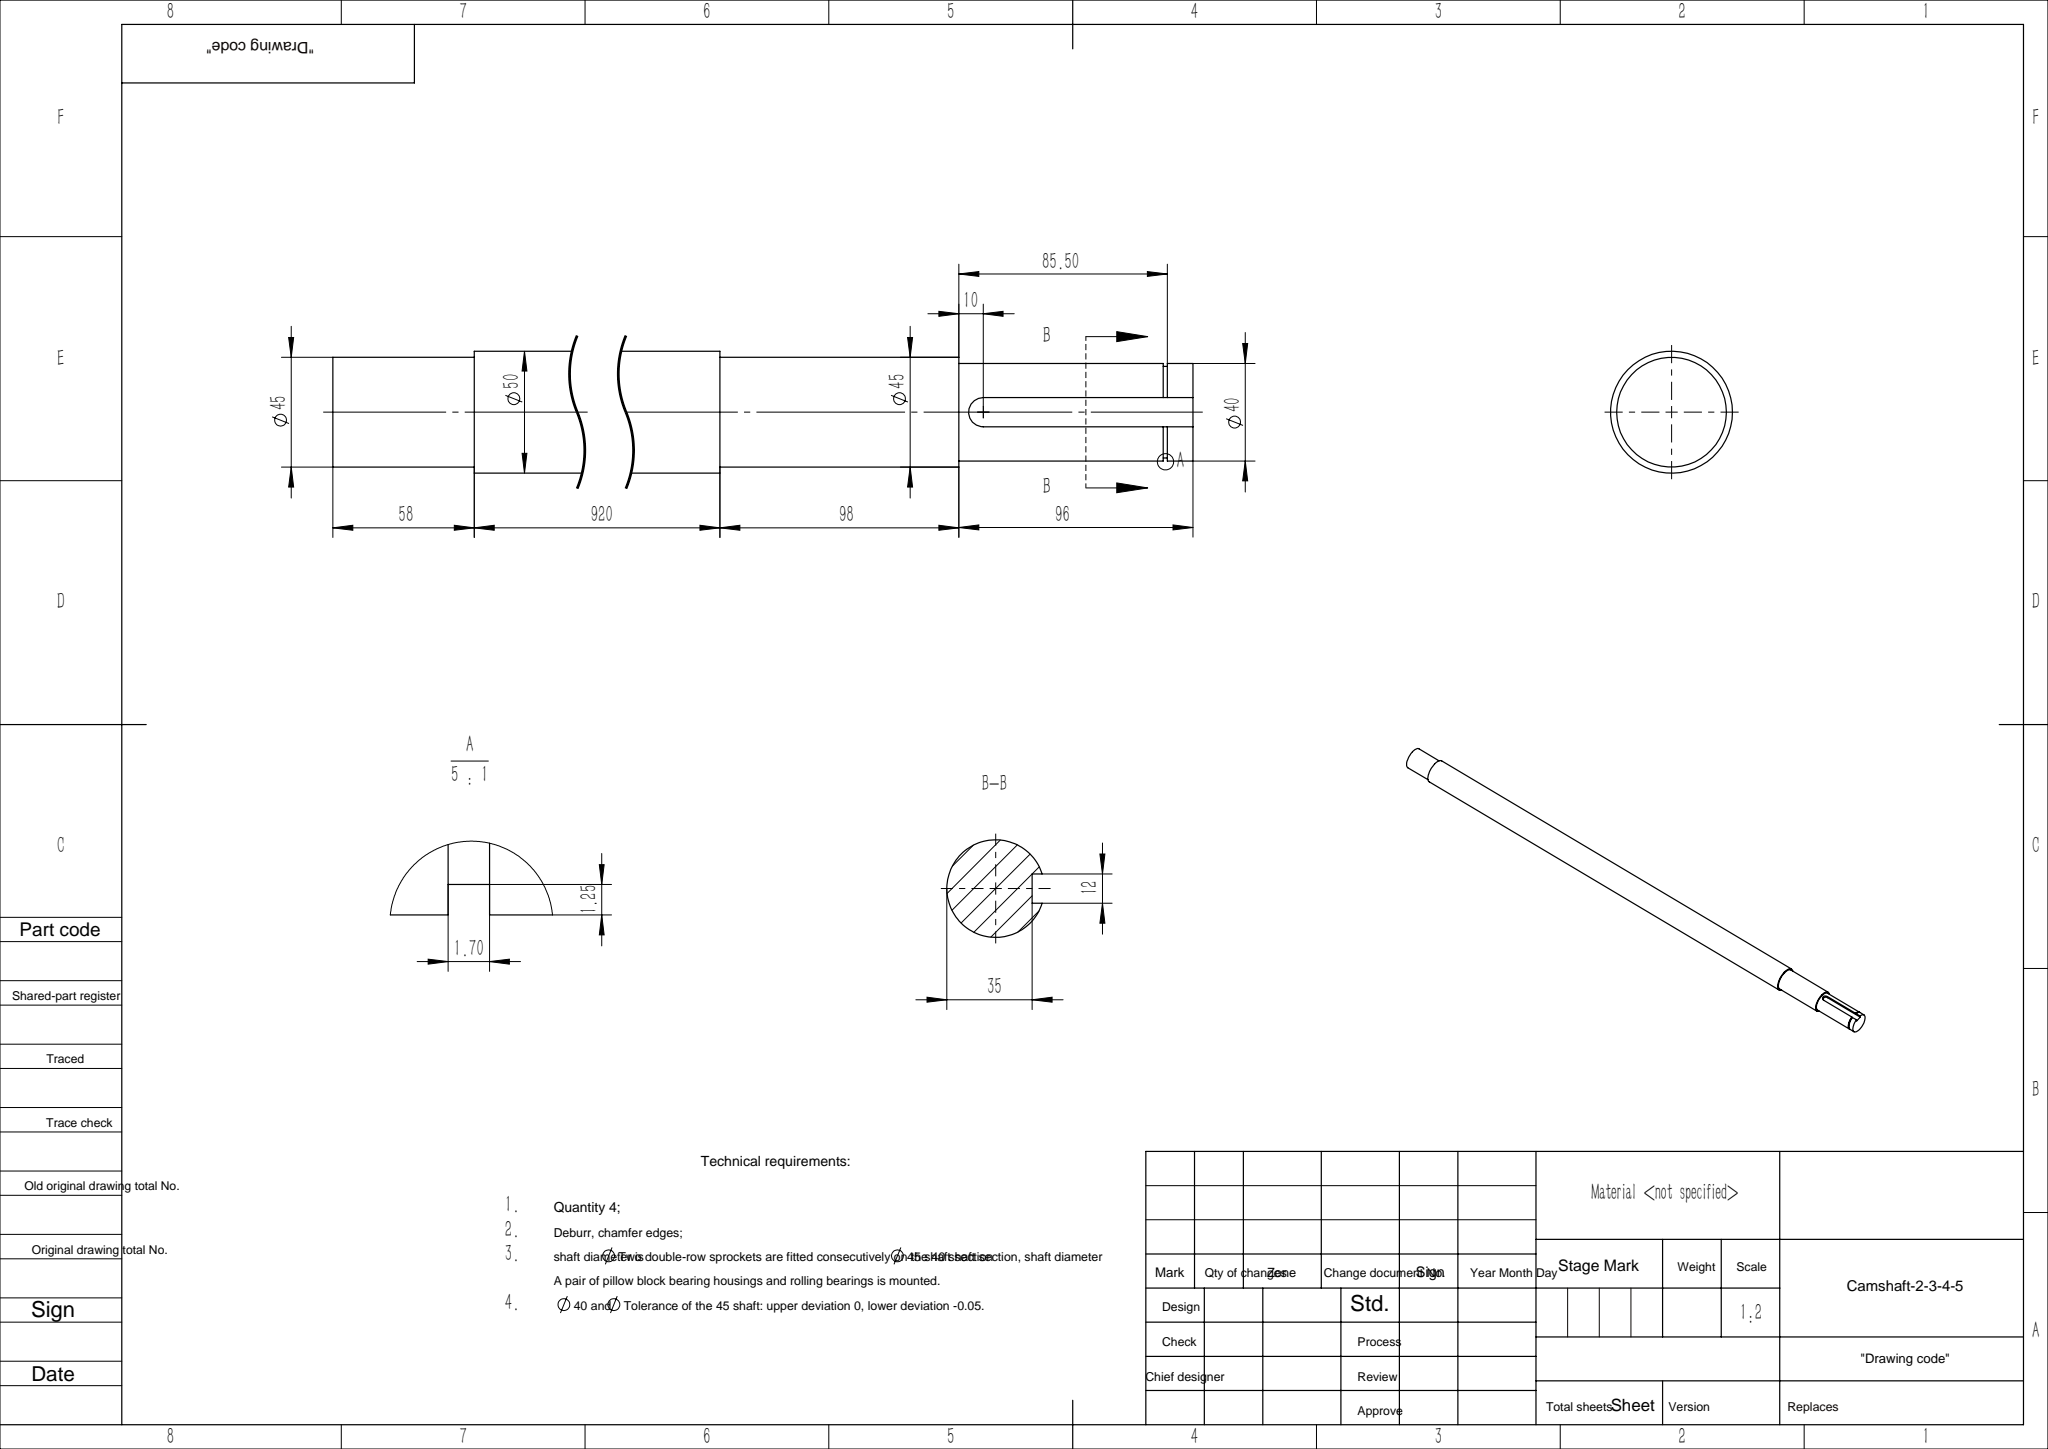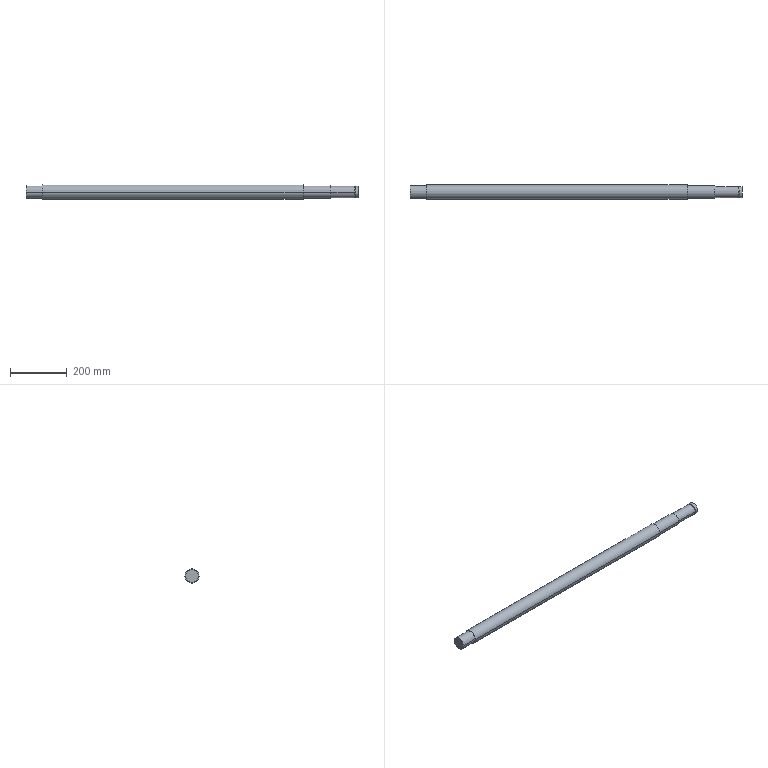Part | SolidWorks | features ICE 2, Revolution 1 | 1 solid | 22 faces | box 1172 x 50 x 50 mm | volume 2169811 mm3 | cylinder 12 | plane 10 | commonest cylinder face diameters 45 x4 40 x3 12 x2 50 x2 37.5 x1
STEP:
#1=CARTESIAN_POINT('',(1080.,15.,0.));
#2=VERTEX_POINT('',#1);
#3=CARTESIAN_POINT('',(1086.,15.,6.));
#4=VERTEX_POINT('',#3);
#5=CARTESIAN_POINT('',(1086.,15.,0.));
#6=DIRECTION('',(0.,1.,0.));
#7=DIRECTION('',(-1.,0.,0.));
#8=AXIS2_PLACEMENT_3D('',#5,#6,#7);
#9=CIRCLE('',#8,6.);
#10=EDGE_CURVE('',#2,#4,#9,.T.);
#11=ORIENTED_EDGE('',*,*,#10,.F.);
#12=CARTESIAN_POINT('',(1080.,20.,0.));
#13=VERTEX_POINT('',#12);
#14=CARTESIAN_POINT('',(1080.,15.,0.));
#15=DIRECTION('',(0.,1.,0.));
#16=VECTOR('',#15,1000.);
#17=LINE('',#14,#16);
#18=EDGE_CURVE('',#2,#13,#17,.T.);
#19=ORIENTED_EDGE('',*,*,#18,.T.);
#20=CARTESIAN_POINT('',(1086.,19.079,6.));
#21=VERTEX_POINT('',#20);
#22=CARTESIAN_POINT('',(1080.,20.,0.));
#23=CARTESIAN_POINT('',(1080.,20.,0.3936));
#24=CARTESIAN_POINT('',(1080.04,19.988,0.7934));
#25=CARTESIAN_POINT('',(1080.194,19.942,1.564));
#26=CARTESIAN_POINT('',(1080.308,19.909,1.939));
#27=CARTESIAN_POINT('',(1080.611,19.825,2.668));
#28=CARTESIAN_POINT('',(1080.798,19.774,3.015));
#29=CARTESIAN_POINT('',(1081.123,19.692,3.5));
#30=CARTESIAN_POINT('',(1081.239,19.664,3.657));
#31=CARTESIAN_POINT('',(1081.487,19.605,3.959));
#32=CARTESIAN_POINT('',(1081.62,19.575,4.105));
#33=CARTESIAN_POINT('',(1082.035,19.485,4.52));
#34=CARTESIAN_POINT('',(1082.335,19.425,4.766));
#35=CARTESIAN_POINT('',(1082.982,19.313,5.201));
#36=CARTESIAN_POINT('',(1083.333,19.261,5.389));
#37=CARTESIAN_POINT('',(1084.055,19.174,5.69));
#38=CARTESIAN_POINT('',(1084.429,19.139,5.804));
#39=CARTESIAN_POINT('',(1085.203,19.092,5.96));
#40=CARTESIAN_POINT('',(1085.601,19.079,6.));
#41=CARTESIAN_POINT('',(1086.,19.079,6.));
#42=B_SPLINE_CURVE_WITH_KNOTS('',3,(#22,#23,#24,#25,#26,#27,#28,#29,#30,#31,#32,#33,#34,#35,#36,#37,#38,#39,#40,#41),.UNSPECIFIED.,.F.,.F.,(4,2,2,2,2,2,2,2,2,4),(0.009436,0.01061,0.01179,0.01297,0.01356,0.01415,0.01533,0.0165,0.01768,0.01886),.UNSPECIFIED.);
#43=EDGE_CURVE('',#13,#21,#42,.T.);
#44=ORIENTED_EDGE('',*,*,#43,.T.);
#45=CARTESIAN_POINT('',(1086.,15.,6.));
#46=DIRECTION('',(0.,1.,0.));
#47=VECTOR('',#46,1000.);
#48=LINE('',#45,#47);
#49=EDGE_CURVE('',#4,#21,#48,.T.);
#50=ORIENTED_EDGE('',*,*,#49,.F.);
#51=EDGE_LOOP('',(#11,#19,#44,#50));
#52=FACE_OUTER_BOUND('',#51,.T.);
#53=CARTESIAN_POINT('',(1086.,15.,0.));
#54=DIRECTION('',(0.,1.,0.));
#55=DIRECTION('',(-1.,0.,0.));
#56=AXIS2_PLACEMENT_3D('',#53,#54,#55);
#57=CYLINDRICAL_SURFACE('',#56,6.);
#58=ADVANCED_FACE('',(#52),#57,.F.);
#59=CARTESIAN_POINT('',(978.,22.5,0.));
#60=VERTEX_POINT('',#59);
#61=CARTESIAN_POINT('',(978.,-22.5,0.));
#62=VERTEX_POINT('',#61);
#63=CARTESIAN_POINT('',(978.,0.,0.));
#64=DIRECTION('',(1.,0.,0.));
#65=DIRECTION('',(0.,1.,0.));
#66=AXIS2_PLACEMENT_3D('',#63,#64,#65);
#67=CIRCLE('',#66,22.5);
#68=EDGE_CURVE('',#60,#62,#67,.T.);
#69=ORIENTED_EDGE('',*,*,#68,.T.);
#70=CARTESIAN_POINT('',(1076.,-22.5,0.));
#71=VERTEX_POINT('',#70);
#72=CARTESIAN_POINT('',(1172.,-22.5,0.));
#73=DIRECTION('',(1.,0.,0.));
#74=VECTOR('',#73,1000.);
#75=LINE('',#72,#74);
#76=EDGE_CURVE('',#62,#71,#75,.T.);
#77=ORIENTED_EDGE('',*,*,#76,.T.);
#78=CARTESIAN_POINT('',(1076.,22.5,0.));
#79=VERTEX_POINT('',#78);
#80=CARTESIAN_POINT('',(1076.,0.,0.));
#81=DIRECTION('',(1.,0.,0.));
#82=DIRECTION('',(0.,1.,0.));
#83=AXIS2_PLACEMENT_3D('',#80,#81,#82);
#84=CIRCLE('',#83,22.5);
#85=EDGE_CURVE('',#79,#71,#84,.T.);
#86=ORIENTED_EDGE('',*,*,#85,.F.);
#87=CARTESIAN_POINT('',(1172.,22.5,0.));
#88=DIRECTION('',(1.,0.,0.));
#89=VECTOR('',#88,1000.);
#90=LINE('',#87,#89);
#91=EDGE_CURVE('',#60,#79,#90,.T.);
#92=ORIENTED_EDGE('',*,*,#91,.F.);
#93=EDGE_LOOP('',(#69,#77,#86,#92));
#94=FACE_OUTER_BOUND('',#93,.T.);
#95=CARTESIAN_POINT('',(1172.,0.,0.));
#96=DIRECTION('',(1.,0.,0.));
#97=DIRECTION('',(0.,1.,0.));
#98=AXIS2_PLACEMENT_3D('',#95,#96,#97);
#99=CYLINDRICAL_SURFACE('',#98,22.5);
#100=ADVANCED_FACE('',(#94),#99,.T.);
#101=CARTESIAN_POINT('',(58.,25.,0.));
#102=VERTEX_POINT('',#101);
#103=CARTESIAN_POINT('',(58.,-25.,0.));
#104=VERTEX_POINT('',#103);
#105=CARTESIAN_POINT('',(58.,0.,0.));
#106=DIRECTION('',(1.,0.,0.));
#107=DIRECTION('',(0.,1.,0.));
#108=AXIS2_PLACEMENT_3D('',#105,#106,#107);
#109=CIRCLE('',#108,25.);
#110=EDGE_CURVE('',#102,#104,#109,.T.);
#111=ORIENTED_EDGE('',*,*,#110,.T.);
#112=CARTESIAN_POINT('',(978.,-25.,0.));
#113=VERTEX_POINT('',#112);
#114=CARTESIAN_POINT('',(1172.,-25.,0.));
#115=DIRECTION('',(1.,0.,0.));
#116=VECTOR('',#115,1000.);
#117=LINE('',#114,#116);
#118=EDGE_CURVE('',#104,#113,#117,.T.);
#119=ORIENTED_EDGE('',*,*,#118,.T.);
#120=CARTESIAN_POINT('',(978.,25.,0.));
#121=VERTEX_POINT('',#120);
#122=CARTESIAN_POINT('',(978.,0.,0.));
#123=DIRECTION('',(1.,0.,0.));
#124=DIRECTION('',(0.,1.,0.));
#125=AXIS2_PLACEMENT_3D('',#122,#123,#124);
#126=CIRCLE('',#125,25.);
#127=EDGE_CURVE('',#121,#113,#126,.T.);
#128=ORIENTED_EDGE('',*,*,#127,.F.);
#129=CARTESIAN_POINT('',(1172.,25.,0.));
#130=DIRECTION('',(1.,0.,0.));
#131=VECTOR('',#130,1000.);
#132=LINE('',#129,#131);
#133=EDGE_CURVE('',#102,#121,#132,.T.);
#134=ORIENTED_EDGE('',*,*,#133,.F.);
#135=EDGE_LOOP('',(#111,#119,#128,#134));
#136=FACE_OUTER_BOUND('',#135,.T.);
#137=CARTESIAN_POINT('',(1172.,0.,0.));
#138=DIRECTION('',(1.,0.,0.));
#139=DIRECTION('',(0.,1.,0.));
#140=AXIS2_PLACEMENT_3D('',#137,#138,#139);
#141=CYLINDRICAL_SURFACE('',#140,25.);
#142=ADVANCED_FACE('',(#136),#141,.T.);
#143=CARTESIAN_POINT('',(0.,22.5,0.));
#144=VERTEX_POINT('',#143);
#145=CARTESIAN_POINT('',(0.,-22.5,0.));
#146=VERTEX_POINT('',#145);
#147=CARTESIAN_POINT('',(0.,0.,0.));
#148=DIRECTION('',(1.,0.,0.));
#149=DIRECTION('',(0.,1.,0.));
#150=AXIS2_PLACEMENT_3D('',#147,#148,#149);
#151=CIRCLE('',#150,22.5);
#152=EDGE_CURVE('',#144,#146,#151,.T.);
#153=ORIENTED_EDGE('',*,*,#152,.T.);
#154=CARTESIAN_POINT('',(58.,-22.5,0.));
#155=VERTEX_POINT('',#154);
#156=CARTESIAN_POINT('',(1172.,-22.5,0.));
#157=DIRECTION('',(1.,0.,0.));
#158=VECTOR('',#157,1000.);
#159=LINE('',#156,#158);
#160=EDGE_CURVE('',#146,#155,#159,.T.);
#161=ORIENTED_EDGE('',*,*,#160,.T.);
#162=CARTESIAN_POINT('',(58.,22.5,0.));
#163=VERTEX_POINT('',#162);
#164=CARTESIAN_POINT('',(58.,0.,0.));
#165=DIRECTION('',(1.,0.,0.));
#166=DIRECTION('',(0.,1.,0.));
#167=AXIS2_PLACEMENT_3D('',#164,#165,#166);
#168=CIRCLE('',#167,22.5);
#169=EDGE_CURVE('',#163,#155,#168,.T.);
#170=ORIENTED_EDGE('',*,*,#169,.F.);
#171=CARTESIAN_POINT('',(1172.,22.5,0.));
#172=DIRECTION('',(1.,0.,0.));
#173=VECTOR('',#172,1000.);
#174=LINE('',#171,#173);
#175=EDGE_CURVE('',#144,#163,#174,.T.);
#176=ORIENTED_EDGE('',*,*,#175,.F.);
#177=EDGE_LOOP('',(#153,#161,#170,#176));
#178=FACE_OUTER_BOUND('',#177,.T.);
#179=CARTESIAN_POINT('',(1172.,0.,0.));
#180=DIRECTION('',(1.,0.,0.));
#181=DIRECTION('',(0.,1.,0.));
#182=AXIS2_PLACEMENT_3D('',#179,#180,#181);
#183=CYLINDRICAL_SURFACE('',#182,22.5);
#184=ADVANCED_FACE('',(#178),#183,.T.);
#185=CARTESIAN_POINT('',(1076.,20.,0.));
#186=VERTEX_POINT('',#185);
#187=CARTESIAN_POINT('',(1076.,-20.,0.));
#188=VERTEX_POINT('',#187);
#189=CARTESIAN_POINT('',(1076.,0.,0.));
#190=DIRECTION('',(1.,0.,0.));
#191=DIRECTION('',(0.,1.,0.));
#192=AXIS2_PLACEMENT_3D('',#189,#190,#191);
#193=CIRCLE('',#192,20.);
#194=EDGE_CURVE('',#186,#188,#193,.T.);
#195=ORIENTED_EDGE('',*,*,#194,.T.);
#196=CARTESIAN_POINT('',(1159.8,-20.,0.));
#197=VERTEX_POINT('',#196);
#198=CARTESIAN_POINT('',(1172.,-20.,0.));
#199=DIRECTION('',(1.,0.,0.));
#200=VECTOR('',#199,1000.);
#201=LINE('',#198,#200);
#202=EDGE_CURVE('',#188,#197,#201,.T.);
#203=ORIENTED_EDGE('',*,*,#202,.T.);
#204=CARTESIAN_POINT('',(1159.8,19.079,6.));
#205=VERTEX_POINT('',#204);
#206=CARTESIAN_POINT('',(1159.8,0.,0.));
#207=DIRECTION('',(1.,0.,0.));
#208=DIRECTION('',(0.,1.,0.));
#209=AXIS2_PLACEMENT_3D('',#206,#207,#208);
#210=CIRCLE('',#209,20.);
#211=EDGE_CURVE('',#205,#197,#210,.T.);
#212=ORIENTED_EDGE('',*,*,#211,.F.);
#213=CARTESIAN_POINT('',(1172.,19.079,6.));
#214=DIRECTION('',(1.,0.,0.));
#215=VECTOR('',#214,1000.);
#216=LINE('',#213,#215);
#217=EDGE_CURVE('',#21,#205,#216,.T.);
#218=ORIENTED_EDGE('',*,*,#217,.F.);
#219=ORIENTED_EDGE('',*,*,#43,.F.);
#220=CARTESIAN_POINT('',(1172.,20.,0.));
#221=DIRECTION('',(1.,0.,0.));
#222=VECTOR('',#221,1000.);
#223=LINE('',#220,#222);
#224=EDGE_CURVE('',#186,#13,#223,.T.);
#225=ORIENTED_EDGE('',*,*,#224,.F.);
#226=EDGE_LOOP('',(#195,#203,#212,#218,#219,#225));
#227=FACE_OUTER_BOUND('',#226,.T.);
#228=CARTESIAN_POINT('',(1172.,0.,0.));
#229=DIRECTION('',(1.,0.,0.));
#230=DIRECTION('',(0.,1.,0.));
#231=AXIS2_PLACEMENT_3D('',#228,#229,#230);
#232=CYLINDRICAL_SURFACE('',#231,20.);
#233=ADVANCED_FACE('',(#227),#232,.T.);
#234=ORIENTED_EDGE('',*,*,#202,.F.);
#235=CARTESIAN_POINT('',(1076.,0.,0.));
#236=DIRECTION('',(1.,0.,0.));
#237=DIRECTION('',(0.,1.,0.));
#238=AXIS2_PLACEMENT_3D('',#235,#236,#237);
#239=CIRCLE('',#238,20.);
#240=EDGE_CURVE('',#188,#186,#239,.T.);
#241=ORIENTED_EDGE('',*,*,#240,.T.);
#242=ORIENTED_EDGE('',*,*,#224,.T.);
#243=CARTESIAN_POINT('',(1086.,19.079,-6.));
#244=VERTEX_POINT('',#243);
#245=CARTESIAN_POINT('',(1086.,19.079,-6.));
#246=CARTESIAN_POINT('',(1085.601,19.079,-6.));
#247=CARTESIAN_POINT('',(1085.209,19.091,-5.961));
#248=CARTESIAN_POINT('',(1084.631,19.127,-5.845));
#249=CARTESIAN_POINT('',(1084.441,19.141,-5.797));
#250=CARTESIAN_POINT('',(1084.062,19.176,-5.682));
#251=CARTESIAN_POINT('',(1083.875,19.196,-5.615));
#252=CARTESIAN_POINT('',(1083.331,19.261,-5.388));
#253=CARTESIAN_POINT('',(1082.987,19.313,-5.203));
#254=CARTESIAN_POINT('',(1082.499,19.397,-4.877));
#255=CARTESIAN_POINT('',(1082.34,19.426,-4.759));
#256=CARTESIAN_POINT('',(1082.037,19.485,-4.51));
#257=CARTESIAN_POINT('',(1081.893,19.515,-4.378));
#258=CARTESIAN_POINT('',(1081.481,19.605,-3.966));
#259=CARTESIAN_POINT('',(1081.233,19.664,-3.665));
#260=CARTESIAN_POINT('',(1080.794,19.775,-3.009));
#261=CARTESIAN_POINT('',(1080.609,19.825,-2.664));
#262=CARTESIAN_POINT('',(1080.385,19.888,-2.122));
#263=CARTESIAN_POINT('',(1080.318,19.907,-1.938));
#264=CARTESIAN_POINT('',(1080.203,19.94,-1.561));
#265=CARTESIAN_POINT('',(1080.154,19.954,-1.367));
#266=CARTESIAN_POINT('',(1080.038,19.988,-0.7852));
#267=CARTESIAN_POINT('',(1080.,20.,-0.3941));
#268=CARTESIAN_POINT('',(1080.,20.,0.));
#269=B_SPLINE_CURVE_WITH_KNOTS('',3,(#245,#246,#247,#248,#249,#250,#251,#252,#253,#254,#255,#256,#257,#258,#259,#260,#261,#262,#263,#264,#265,#266,#267,#268),.UNSPECIFIED.,.F.,.F.,(4,2,2,2,2,2,2,2,2,2,2,4),(0.,0.00118,0.001769,0.002359,0.003539,0.004128,0.004718,0.005898,0.007077,0.007667,0.008257,0.009436),.UNSPECIFIED.);
#270=EDGE_CURVE('',#244,#13,#269,.T.);
#271=ORIENTED_EDGE('',*,*,#270,.F.);
#272=CARTESIAN_POINT('',(1159.8,19.079,-6.));
#273=VERTEX_POINT('',#272);
#274=CARTESIAN_POINT('',(1172.,19.079,-6.));
#275=DIRECTION('',(-1.,0.,0.));
#276=VECTOR('',#275,1000.);
#277=LINE('',#274,#276);
#278=EDGE_CURVE('',#273,#244,#277,.T.);
#279=ORIENTED_EDGE('',*,*,#278,.F.);
#280=CARTESIAN_POINT('',(1159.8,0.,0.));
#281=DIRECTION('',(1.,0.,0.));
#282=DIRECTION('',(0.,1.,0.));
#283=AXIS2_PLACEMENT_3D('',#280,#281,#282);
#284=CIRCLE('',#283,20.);
#285=EDGE_CURVE('',#197,#273,#284,.T.);
#286=ORIENTED_EDGE('',*,*,#285,.F.);
#287=EDGE_LOOP('',(#234,#241,#242,#271,#279,#286));
#288=FACE_OUTER_BOUND('',#287,.T.);
#289=CARTESIAN_POINT('',(1172.,0.,0.));
#290=DIRECTION('',(1.,0.,0.));
#291=DIRECTION('',(0.,1.,0.));
#292=AXIS2_PLACEMENT_3D('',#289,#290,#291);
#293=CYLINDRICAL_SURFACE('',#292,20.);
#294=ADVANCED_FACE('',(#288),#293,.T.);
#295=CARTESIAN_POINT('',(1159.8,17.764,-6.));
#296=VERTEX_POINT('',#295);
#297=CARTESIAN_POINT('',(1159.8,15.,-6.));
#298=DIRECTION('',(0.,-1.,0.));
#299=VECTOR('',#298,1000.);
#300=LINE('',#297,#299);
#301=EDGE_CURVE('',#273,#296,#300,.T.);
#302=ORIENTED_EDGE('',*,*,#301,.F.);
#303=ORIENTED_EDGE('',*,*,#278,.T.);
#304=CARTESIAN_POINT('',(1086.,15.,-6.));
#305=VERTEX_POINT('',#304);
#306=CARTESIAN_POINT('',(1086.,15.,-6.));
#307=DIRECTION('',(0.,1.,0.));
#308=VECTOR('',#307,1000.);
#309=LINE('',#306,#308);
#310=EDGE_CURVE('',#305,#244,#309,.T.);
#311=ORIENTED_EDGE('',*,*,#310,.F.);
#312=CARTESIAN_POINT('',(1172.,15.,-6.));
#313=VERTEX_POINT('',#312);
#314=CARTESIAN_POINT('',(1086.,15.,-6.));
#315=DIRECTION('',(-1.,0.,0.));
#316=VECTOR('',#315,1000.);
#317=LINE('',#314,#316);
#318=EDGE_CURVE('',#313,#305,#317,.T.);
#319=ORIENTED_EDGE('',*,*,#318,.F.);
#320=CARTESIAN_POINT('',(1172.,19.079,-6.));
#321=VERTEX_POINT('',#320);
#322=CARTESIAN_POINT('',(1172.,20.,-6.));
#323=DIRECTION('',(0.,1.,0.));
#324=VECTOR('',#323,1000.);
#325=LINE('',#322,#324);
#326=EDGE_CURVE('',#313,#321,#325,.T.);
#327=ORIENTED_EDGE('',*,*,#326,.T.);
#328=CARTESIAN_POINT('',(1161.5,19.079,-6.));
#329=VERTEX_POINT('',#328);
#330=CARTESIAN_POINT('',(1172.,19.079,-6.));
#331=DIRECTION('',(-1.,0.,0.));
#332=VECTOR('',#331,1000.);
#333=LINE('',#330,#332);
#334=EDGE_CURVE('',#321,#329,#333,.T.);
#335=ORIENTED_EDGE('',*,*,#334,.T.);
#336=CARTESIAN_POINT('',(1161.5,17.764,-6.));
#337=VERTEX_POINT('',#336);
#338=CARTESIAN_POINT('',(1161.5,15.,-6.));
#339=DIRECTION('',(0.,-1.,0.));
#340=VECTOR('',#339,1000.);
#341=LINE('',#338,#340);
#342=EDGE_CURVE('',#329,#337,#341,.T.);
#343=ORIENTED_EDGE('',*,*,#342,.T.);
#344=CARTESIAN_POINT('',(1159.8,17.764,-6.));
#345=DIRECTION('',(1.,0.,0.));
#346=VECTOR('',#345,1000.);
#347=LINE('',#344,#346);
#348=EDGE_CURVE('',#296,#337,#347,.T.);
#349=ORIENTED_EDGE('',*,*,#348,.F.);
#350=EDGE_LOOP('',(#302,#303,#311,#319,#327,#335,#343,#349));
#351=FACE_OUTER_BOUND('',#350,.T.);
#352=CARTESIAN_POINT('',(1086.,15.,-6.));
#353=DIRECTION('',(0.,0.,-1.));
#354=DIRECTION('',(-1.,0.,0.));
#355=AXIS2_PLACEMENT_3D('',#352,#353,#354);
#356=PLANE('',#355);
#357=ADVANCED_FACE('',(#351),#356,.F.);
#358=CARTESIAN_POINT('',(1159.8,17.764,6.));
#359=VERTEX_POINT('',#358);
#360=CARTESIAN_POINT('',(1159.8,15.,6.));
#361=DIRECTION('',(0.,1.,0.));
#362=VECTOR('',#361,1000.);
#363=LINE('',#360,#362);
#364=EDGE_CURVE('',#359,#205,#363,.T.);
#365=ORIENTED_EDGE('',*,*,#364,.F.);
#366=CARTESIAN_POINT('',(1161.5,17.764,6.));
#367=VERTEX_POINT('',#366);
#368=CARTESIAN_POINT('',(1159.8,17.764,6.));
#369=DIRECTION('',(-1.,0.,0.));
#370=VECTOR('',#369,1000.);
#371=LINE('',#368,#370);
#372=EDGE_CURVE('',#367,#359,#371,.T.);
#373=ORIENTED_EDGE('',*,*,#372,.F.);
#374=CARTESIAN_POINT('',(1161.5,19.079,6.));
#375=VERTEX_POINT('',#374);
#376=CARTESIAN_POINT('',(1161.5,15.,6.));
#377=DIRECTION('',(0.,1.,0.));
#378=VECTOR('',#377,1000.);
#379=LINE('',#376,#378);
#380=EDGE_CURVE('',#367,#375,#379,.T.);
#381=ORIENTED_EDGE('',*,*,#380,.T.);
#382=CARTESIAN_POINT('',(1172.,19.079,6.));
#383=VERTEX_POINT('',#382);
#384=CARTESIAN_POINT('',(1172.,19.079,6.));
#385=DIRECTION('',(1.,0.,0.));
#386=VECTOR('',#385,1000.);
#387=LINE('',#384,#386);
#388=EDGE_CURVE('',#375,#383,#387,.T.);
#389=ORIENTED_EDGE('',*,*,#388,.T.);
#390=CARTESIAN_POINT('',(1172.,15.,6.));
#391=VERTEX_POINT('',#390);
#392=CARTESIAN_POINT('',(1172.,20.,6.));
#393=DIRECTION('',(0.,-1.,0.));
#394=VECTOR('',#393,1000.);
#395=LINE('',#392,#394);
#396=EDGE_CURVE('',#383,#391,#395,.T.);
#397=ORIENTED_EDGE('',*,*,#396,.T.);
#398=CARTESIAN_POINT('',(1086.,15.,6.));
#399=DIRECTION('',(1.,0.,0.));
#400=VECTOR('',#399,1000.);
#401=LINE('',#398,#400);
#402=EDGE_CURVE('',#4,#391,#401,.T.);
#403=ORIENTED_EDGE('',*,*,#402,.F.);
#404=ORIENTED_EDGE('',*,*,#49,.T.);
#405=ORIENTED_EDGE('',*,*,#217,.T.);
#406=EDGE_LOOP('',(#365,#373,#381,#389,#397,#403,#404,#405));
#407=FACE_OUTER_BOUND('',#406,.T.);
#408=CARTESIAN_POINT('',(1086.,15.,6.));
#409=DIRECTION('',(0.,0.,1.));
#410=DIRECTION('',(1.,0.,0.));
#411=AXIS2_PLACEMENT_3D('',#408,#409,#410);
#412=PLANE('',#411);
#413=ADVANCED_FACE('',(#407),#412,.F.);
#414=ORIENTED_EDGE('',*,*,#152,.F.);
#415=CARTESIAN_POINT('',(0.,0.,0.));
#416=DIRECTION('',(1.,0.,0.));
#417=DIRECTION('',(0.,1.,0.));
#418=AXIS2_PLACEMENT_3D('',#415,#416,#417);
#419=CIRCLE('',#418,22.5);
#420=EDGE_CURVE('',#146,#144,#419,.T.);
#421=ORIENTED_EDGE('',*,*,#420,.F.);
#422=EDGE_LOOP('',(#414,#421));
#423=FACE_OUTER_BOUND('',#422,.T.);
#424=CARTESIAN_POINT('',(0.,0.,0.));
#425=DIRECTION('',(-1.,0.,0.));
#426=DIRECTION('',(0.,-1.,0.));
#427=AXIS2_PLACEMENT_3D('',#424,#425,#426);
#428=PLANE('',#427);
#429=ADVANCED_FACE('',(#423),#428,.T.);
#430=ORIENTED_EDGE('',*,*,#160,.F.);
#431=ORIENTED_EDGE('',*,*,#420,.T.);
#432=ORIENTED_EDGE('',*,*,#175,.T.);
#433=CARTESIAN_POINT('',(58.,0.,0.));
#434=DIRECTION('',(1.,0.,0.));
#435=DIRECTION('',(0.,1.,0.));
#436=AXIS2_PLACEMENT_3D('',#433,#434,#435);
#437=CIRCLE('',#436,22.5);
#438=EDGE_CURVE('',#155,#163,#437,.T.);
#439=ORIENTED_EDGE('',*,*,#438,.F.);
#440=EDGE_LOOP('',(#430,#431,#432,#439));
#441=FACE_OUTER_BOUND('',#440,.T.);
#442=CARTESIAN_POINT('',(1172.,0.,0.));
#443=DIRECTION('',(1.,0.,0.));
#444=DIRECTION('',(0.,1.,0.));
#445=AXIS2_PLACEMENT_3D('',#442,#443,#444);
#446=CYLINDRICAL_SURFACE('',#445,22.5);
#447=ADVANCED_FACE('',(#441),#446,.T.);
#448=ORIENTED_EDGE('',*,*,#169,.T.);
#449=ORIENTED_EDGE('',*,*,#438,.T.);
#450=EDGE_LOOP('',(#448,#449));
#451=FACE_BOUND('',#450,.T.);
#452=ORIENTED_EDGE('',*,*,#110,.F.);
#453=CARTESIAN_POINT('',(58.,0.,0.));
#454=DIRECTION('',(1.,0.,0.));
#455=DIRECTION('',(0.,1.,0.));
#456=AXIS2_PLACEMENT_3D('',#453,#454,#455);
#457=CIRCLE('',#456,25.);
#458=EDGE_CURVE('',#104,#102,#457,.T.);
#459=ORIENTED_EDGE('',*,*,#458,.F.);
#460=EDGE_LOOP('',(#452,#459));
#461=FACE_OUTER_BOUND('',#460,.T.);
#462=CARTESIAN_POINT('',(58.,22.5,0.));
#463=DIRECTION('',(-1.,0.,0.));
#464=DIRECTION('',(0.,-1.,0.));
#465=AXIS2_PLACEMENT_3D('',#462,#463,#464);
#466=PLANE('',#465);
#467=ADVANCED_FACE('',(#451,#461),#466,.T.);
#468=ORIENTED_EDGE('',*,*,#118,.F.);
#469=ORIENTED_EDGE('',*,*,#458,.T.);
#470=ORIENTED_EDGE('',*,*,#133,.T.);
#471=CARTESIAN_POINT('',(978.,0.,0.));
#472=DIRECTION('',(1.,0.,0.));
#473=DIRECTION('',(0.,1.,0.));
#474=AXIS2_PLACEMENT_3D('',#471,#472,#473);
#475=CIRCLE('',#474,25.);
#476=EDGE_CURVE('',#113,#121,#475,.T.);
#477=ORIENTED_EDGE('',*,*,#476,.F.);
#478=EDGE_LOOP('',(#468,#469,#470,#477));
#479=FACE_OUTER_BOUND('',#478,.T.);
#480=CARTESIAN_POINT('',(1172.,0.,0.));
#481=DIRECTION('',(1.,0.,0.));
#482=DIRECTION('',(0.,1.,0.));
#483=AXIS2_PLACEMENT_3D('',#480,#481,#482);
#484=CYLINDRICAL_SURFACE('',#483,25.);
#485=ADVANCED_FACE('',(#479),#484,.T.);
#486=ORIENTED_EDGE('',*,*,#127,.T.);
#487=ORIENTED_EDGE('',*,*,#476,.T.);
#488=EDGE_LOOP('',(#486,#487));
#489=FACE_OUTER_BOUND('',#488,.T.);
#490=ORIENTED_EDGE('',*,*,#68,.F.);
#491=CARTESIAN_POINT('',(978.,0.,0.));
#492=DIRECTION('',(1.,0.,0.));
#493=DIRECTION('',(0.,1.,0.));
#494=AXIS2_PLACEMENT_3D('',#491,#492,#493);
#495=CIRCLE('',#494,22.5);
#496=EDGE_CURVE('',#62,#60,#495,.T.);
#497=ORIENTED_EDGE('',*,*,#496,.F.);
#498=EDGE_LOOP('',(#490,#497));
#499=FACE_BOUND('',#498,.T.);
#500=CARTESIAN_POINT('',(978.,25.,0.));
#501=DIRECTION('',(1.,0.,0.));
#502=DIRECTION('',(0.,1.,0.));
#503=AXIS2_PLACEMENT_3D('',#500,#501,#502);
#504=PLANE('',#503);
#505=ADVANCED_FACE('',(#489,#499),#504,.T.);
#506=ORIENTED_EDGE('',*,*,#76,.F.);
#507=ORIENTED_EDGE('',*,*,#496,.T.);
#508=ORIENTED_EDGE('',*,*,#91,.T.);
#509=CARTESIAN_POINT('',(1076.,0.,0.));
#510=DIRECTION('',(1.,0.,0.));
#511=DIRECTION('',(0.,1.,0.));
#512=AXIS2_PLACEMENT_3D('',#509,#510,#511);
#513=CIRCLE('',#512,22.5);
#514=EDGE_CURVE('',#71,#79,#513,.T.);
#515=ORIENTED_EDGE('',*,*,#514,.F.);
#516=EDGE_LOOP('',(#506,#507,#508,#515));
#517=FACE_OUTER_BOUND('',#516,.T.);
#518=CARTESIAN_POINT('',(1172.,0.,0.));
#519=DIRECTION('',(1.,0.,0.));
#520=DIRECTION('',(0.,1.,0.));
#521=AXIS2_PLACEMENT_3D('',#518,#519,#520);
#522=CYLINDRICAL_SURFACE('',#521,22.5);
#523=ADVANCED_FACE('',(#517),#522,.T.);
#524=ORIENTED_EDGE('',*,*,#85,.T.);
#525=ORIENTED_EDGE('',*,*,#514,.T.);
#526=EDGE_LOOP('',(#524,#525));
#527=FACE_OUTER_BOUND('',#526,.T.);
#528=ORIENTED_EDGE('',*,*,#194,.F.);
#529=ORIENTED_EDGE('',*,*,#240,.F.);
#530=EDGE_LOOP('',(#528,#529));
#531=FACE_BOUND('',#530,.T.);
#532=CARTESIAN_POINT('',(1076.,22.5,0.));
#533=DIRECTION('',(1.,0.,0.));
#534=DIRECTION('',(0.,1.,0.));
#535=AXIS2_PLACEMENT_3D('',#532,#533,#534);
#536=PLANE('',#535);
#537=ADVANCED_FACE('',(#527,#531),#536,.T.);
#538=CARTESIAN_POINT('',(1161.5,0.,0.));
#539=DIRECTION('',(1.,0.,0.));
#540=DIRECTION('',(0.,1.,0.));
#541=AXIS2_PLACEMENT_3D('',#538,#539,#540);
#542=CIRCLE('',#541,20.);
#543=EDGE_CURVE('',#375,#329,#542,.T.);
#544=ORIENTED_EDGE('',*,*,#543,.T.);
#545=ORIENTED_EDGE('',*,*,#334,.F.);
#546=CARTESIAN_POINT('',(1172.,0.,0.));
#547=DIRECTION('',(1.,0.,0.));
#548=DIRECTION('',(0.,1.,0.));
#549=AXIS2_PLACEMENT_3D('',#546,#547,#548);
#550=CIRCLE('',#549,20.);
#551=EDGE_CURVE('',#383,#321,#550,.T.);
#552=ORIENTED_EDGE('',*,*,#551,.F.);
#553=ORIENTED_EDGE('',*,*,#388,.F.);
#554=EDGE_LOOP('',(#544,#545,#552,#553));
#555=FACE_OUTER_BOUND('',#554,.T.);
#556=CARTESIAN_POINT('',(1172.,0.,0.));
#557=DIRECTION('',(1.,0.,0.));
#558=DIRECTION('',(0.,1.,0.));
#559=AXIS2_PLACEMENT_3D('',#556,#557,#558);
#560=CYLINDRICAL_SURFACE('',#559,20.);
#561=ADVANCED_FACE('',(#555),#560,.T.);
#562=ORIENTED_EDGE('',*,*,#326,.F.);
#563=CARTESIAN_POINT('',(1172.,15.,0.));
#564=DIRECTION('',(0.,0.,1.));
#565=VECTOR('',#564,1000.);
#566=LINE('',#563,#565);
#567=EDGE_CURVE('',#313,#391,#566,.T.);
#568=ORIENTED_EDGE('',*,*,#567,.T.);
#569=ORIENTED_EDGE('',*,*,#396,.F.);
#570=ORIENTED_EDGE('',*,*,#551,.T.);
#571=EDGE_LOOP('',(#562,#568,#569,#570));
#572=FACE_OUTER_BOUND('',#571,.T.);
#573=CARTESIAN_POINT('',(1172.,20.,0.));
#574=DIRECTION('',(1.,0.,0.));
#575=DIRECTION('',(0.,1.,0.));
#576=AXIS2_PLACEMENT_3D('',#573,#574,#575);
#577=PLANE('',#576);
#578=ADVANCED_FACE('',(#572),#577,.T.);
#579=ORIENTED_EDGE('',*,*,#18,.F.);
#580=CARTESIAN_POINT('',(1086.,15.,0.));
#581=DIRECTION('',(0.,1.,0.));
#582=DIRECTION('',(-1.,0.,0.));
#583=AXIS2_PLACEMENT_3D('',#580,#581,#582);
#584=CIRCLE('',#583,6.);
#585=EDGE_CURVE('',#305,#2,#584,.T.);
#586=ORIENTED_EDGE('',*,*,#585,.F.);
#587=ORIENTED_EDGE('',*,*,#310,.T.);
#588=ORIENTED_EDGE('',*,*,#270,.T.);
#589=EDGE_LOOP('',(#579,#586,#587,#588));
#590=FACE_OUTER_BOUND('',#589,.T.);
#591=CARTESIAN_POINT('',(1086.,15.,0.));
#592=DIRECTION('',(0.,1.,0.));
#593=DIRECTION('',(-1.,0.,0.));
#594=AXIS2_PLACEMENT_3D('',#591,#592,#593);
#595=CYLINDRICAL_SURFACE('',#594,6.);
#596=ADVANCED_FACE('',(#590),#595,.F.);
#597=ORIENTED_EDGE('',*,*,#318,.T.);
#598=ORIENTED_EDGE('',*,*,#585,.T.);
#599=ORIENTED_EDGE('',*,*,#10,.T.);
#600=ORIENTED_EDGE('',*,*,#402,.T.);
#601=ORIENTED_EDGE('',*,*,#567,.F.);
#602=EDGE_LOOP('',(#597,#598,#599,#600,#601));
#603=FACE_OUTER_BOUND('',#602,.T.);
#604=CARTESIAN_POINT('',(1086.,15.,0.));
#605=DIRECTION('',(0.,1.,0.));
#606=DIRECTION('',(-1.,0.,0.));
#607=AXIS2_PLACEMENT_3D('',#604,#605,#606);
#608=PLANE('',#607);
#609=ADVANCED_FACE('',(#603),#608,.T.);
#610=ORIENTED_EDGE('',*,*,#301,.T.);
#611=CARTESIAN_POINT('',(1159.8,0.,0.));
#612=DIRECTION('',(1.,0.,0.));
#613=DIRECTION('',(0.,1.,0.));
#614=AXIS2_PLACEMENT_3D('',#611,#612,#613);
#615=CIRCLE('',#614,18.75);
#616=EDGE_CURVE('',#359,#296,#615,.T.);
#617=ORIENTED_EDGE('',*,*,#616,.F.);
#618=ORIENTED_EDGE('',*,*,#364,.T.);
#619=ORIENTED_EDGE('',*,*,#211,.T.);
#620=ORIENTED_EDGE('',*,*,#285,.T.);
#621=EDGE_LOOP('',(#610,#617,#618,#619,#620));
#622=FACE_OUTER_BOUND('',#621,.T.);
#623=CARTESIAN_POINT('',(1159.8,0.,0.));
#624=DIRECTION('',(1.,0.,0.));
#625=DIRECTION('',(0.,1.,0.));
#626=AXIS2_PLACEMENT_3D('',#623,#624,#625);
#627=PLANE('',#626);
#628=ADVANCED_FACE('',(#622),#627,.T.);
#629=ORIENTED_EDGE('',*,*,#543,.F.);
#630=ORIENTED_EDGE('',*,*,#380,.F.);
#631=CARTESIAN_POINT('',(1161.5,0.,0.));
#632=DIRECTION('',(1.,0.,0.));
#633=DIRECTION('',(0.,1.,0.));
#634=AXIS2_PLACEMENT_3D('',#631,#632,#633);
#635=CIRCLE('',#634,18.75);
#636=EDGE_CURVE('',#367,#337,#635,.T.);
#637=ORIENTED_EDGE('',*,*,#636,.T.);
#638=ORIENTED_EDGE('',*,*,#342,.F.);
#639=EDGE_LOOP('',(#629,#630,#637,#638));
#640=FACE_OUTER_BOUND('',#639,.T.);
#641=CARTESIAN_POINT('',(1161.5,0.,0.));
#642=DIRECTION('',(1.,0.,0.));
#643=DIRECTION('',(0.,1.,0.));
#644=AXIS2_PLACEMENT_3D('',#641,#642,#643);
#645=PLANE('',#644);
#646=ADVANCED_FACE('',(#640),#645,.F.);
#647=ORIENTED_EDGE('',*,*,#348,.T.);
#648=ORIENTED_EDGE('',*,*,#636,.F.);
#649=ORIENTED_EDGE('',*,*,#372,.T.);
#650=ORIENTED_EDGE('',*,*,#616,.T.);
#651=EDGE_LOOP('',(#647,#648,#649,#650));
#652=FACE_OUTER_BOUND('',#651,.T.);
#653=CARTESIAN_POINT('',(1159.8,0.,0.));
#654=DIRECTION('',(1.,0.,0.));
#655=DIRECTION('',(0.,1.,0.));
#656=AXIS2_PLACEMENT_3D('',#653,#654,#655);
#657=CYLINDRICAL_SURFACE('',#656,18.75);
#658=ADVANCED_FACE('',(#652),#657,.T.);
#659=CLOSED_SHELL('',(#58,#100,#142,#184,#233,#294,#357,#413,#429,#447,#467,#485,#505,#523,#537,#561,#578,#596,#609,#628,#646,#658));
#660=MANIFOLD_SOLID_BREP('',#659);
#661=CARTESIAN_POINT('',(0.,0.,0.));
#662=DIRECTION('',(0.,0.,1.));
#663=DIRECTION('',(1.,0.,0.));
#664=AXIS2_PLACEMENT_3D('',#661,#662,#663);
#665=(LENGTH_UNIT()NAMED_UNIT(*)SI_UNIT(.MILLI.,.METRE.));
#666=UNCERTAINTY_MEASURE_WITH_UNIT(LENGTH_MEASURE(0.00001),#665,'','');
#667=(NAMED_UNIT(*)PLANE_ANGLE_UNIT()SI_UNIT($,.RADIAN.));
#668=(NAMED_UNIT(*)SI_UNIT($,.STERADIAN.)SOLID_ANGLE_UNIT());
#669=(GEOMETRIC_REPRESENTATION_CONTEXT(3)GLOBAL_UNCERTAINTY_ASSIGNED_CONTEXT((#666))GLOBAL_UNIT_ASSIGNED_CONTEXT((#665,#667,#668))REPRESENTATION_CONTEXT('',''));
#670=ADVANCED_BREP_SHAPE_REPRESENTATION('',(#660,#664),#669);